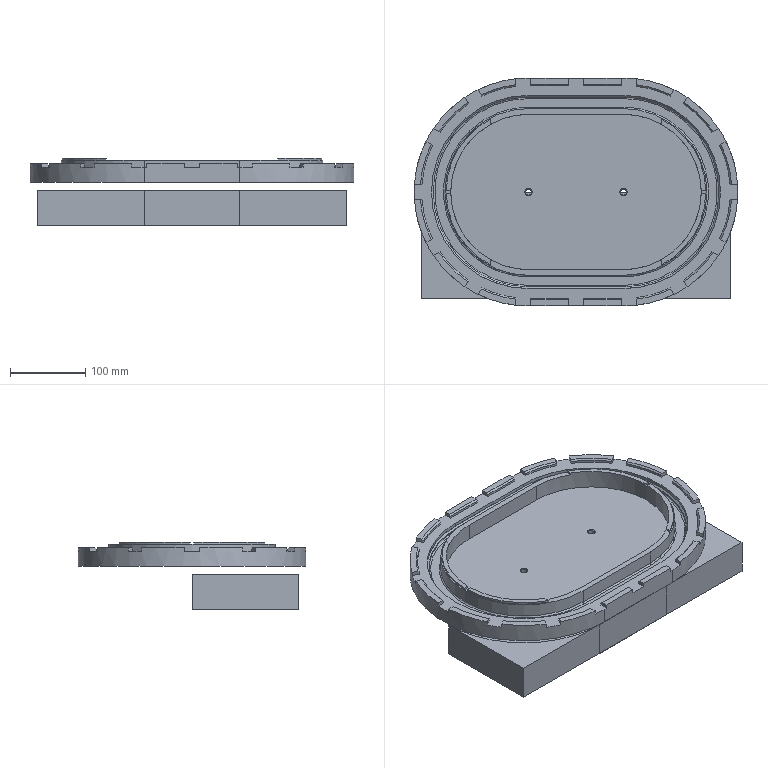NC program | NX | posted with a generic post | part box 429 x 302 x 89.371 mm
Lines 48932 to 50400 of 53366:
(PLANAR_MILL , TOOL : D63.)
N97854 T01 M6
N97856 G53
N97858 G17 G0 G90 X-190.948 Y-133.403 S4500 M3
N97860 G43 Z50. H1
N97862 Z3.1
N97864 G94 G1 Z0.1 F1500.
N97866 X-190.9 Y-70.403
N97868 G2 X-63.5 Y56.9 R127.4
N97870 G1 X63.5
N97872 G2 X190.9 Y-70.403 R127.4
N97874 G1 X190.948 Y-133.403
N97876 Z3.1
N97878 G0 Z50.
N97880 M5
(ADAPTIVE_MILLING_2 , TOOL : D16开粗)
N97882 T02 M6
N97884 G53
N97886 G17 G0 G90 X-224.171 Y-82.61 S6500 M3
N97888 G43 Z50. H2
N97890 Z-47.15
N97892 G94 G1 X-224.022 Y-82.588 Z-48.087 F3000.
N97894 X-223.874 Y-82.566 Z-48.458
N97896 X-223.725 Y-82.545 Z-48.73
N97898 X-223.577 Y-82.523 Z-48.95
N97900 X-223.429 Y-82.501 Z-49.134
N97902 X-223.28 Y-82.479 Z-49.292
N97904 X-223.132 Y-82.457 Z-49.43
N97906 X-222.983 Y-82.435 Z-49.55
N97908 X-222.835 Y-82.413 Z-49.655
N97910 X-222.687 Y-82.392 Z-49.748
N97912 X-222.538 Y-82.37 Z-49.829
N97914 X-222.39 Y-82.348 Z-49.9
N97916 X-222.241 Y-82.326 Z-49.96
N97918 X-222.093 Y-82.304 Z-50.012
N97920 X-221.945 Y-82.282 Z-50.055
N97922 X-221.796 Y-82.26 Z-50.089
N97924 X-221.648 Y-82.238 Z-50.116
N97926 X-221.499 Y-82.217 Z-50.135
N97928 X-221.351 Y-82.195 Z-50.146
N97930 X-221.203 Y-82.173 Z-50.15
N97932 X-218.756 Y-81.812
N97934 G3 X-217.377 Y-80.294 R1.616
N97936 G1 X-217.33 Y-79.346
N97938 G3 X-216.572 Y-73.312 R29.306
N97940 X-216.406 Y-60.427 R336.586
N97942 G1 X-216.401 Y-53.236
N97944 X-216.4 Y71.713
N97946 G2 X-214.045 Y77.327 R8.531
N97948 X-208.506 Y80.787 R13.167
N97950 X-201.742 Y82.057 R28.226
N97952 X-191.324 Y82.379 R143.598
N97954 G1 X-179.699 Y82.399
N97956 X205.701
N97958 G2 X211.373 Y80.002 R8.548
N97960 X214.807 Y74.446 R13.234
N97962 X216.043 Y67.902 R28.051
N97964 X216.374 Y58.01 R132.54
N97966 G1 X216.399 Y45.56
N97968 X216.4 Y-74.626
N97970 G3 X216.43 Y-76.436 R16.956
N97972 G1 X216.538 Y-76.795
N97974 G3 X217.249 Y-77.422 R1.606
N97976 G1 X218.397 Y-77.937
N97978 X221.284 Y-79.232 Z-50.05
N97980 X222.24 Y-79.661 F15000.
N97982 G3 X223.658 Y-76.795 R1.6
N97984 X222.224 Y-76.639 R1.659
N97986 X221.227 Y-77.757 R1.601
N97988 G1 X221.129 Y-78.154
N97990 X220.506 Y-80.674 Z-50.132 F3000.
N97992 G2 X220.252 Y-81.179 Z-50.15 R1.628
N97994 X217.377 Y-80.293 R1.6
N97996 G1 X217.33 Y-79.348
N97998 X217.049 Y-78.058
N98000 G3 X216.45 Y-76.634 R13.354
N98002 G2 X215.994 Y-73.564 R13.236
N98004 X215.806 Y-63.419 R183.776
N98006 G1 X215.8 Y-55.783
N98008 X215.799 Y46.392
N98010 G3 X215.672 Y63.09 R605.854
N98012 X214.951 Y70.698 R48.69
N98014 X213.141 Y75.758 R15.545
N98016 X207.97 Y80.015 R11.123
N98018 X201.787 Y81.461 R20.911
N98020 X193.696 Y81.776 R93.362
N98022 G1 X183.121 Y81.799
N98024 X-183.604 Y81.797
N98026 G3 X-198.002 Y81.638 R400.341
N98028 X-205.298 Y80.826 R42.086
N98030 X-210.087 Y78.934 R14.28
N98032 X-214.129 Y73.746 R11.263
N98034 X-215.472 Y67.766 R21.283
N98036 X-215.78 Y59.45 R97.239
N98038 G1 X-215.8 Y49.7
N98040 X-215.802 Y-55.212
N98042 G2 X-215.933 Y-71.609 R576.074
N98044 X-216.291 Y-76.26 R40.051
N98046 G1 X-216.426 Y-76.609
N98048 G2 X-217.715 Y-77.39 R1.601
N98050 G1 X-218.015 Y-77.379 Z-50.141
N98052 X-218.312 Y-77.339 Z-50.131
N98054 X-220.853 Y-77. Z-50.05
N98056 X-221.994 Y-76.848 F15000.
N98058 G2 X-223.303 Y-74.766 R1.6
N98060 X-223.056 Y-74.152 R2.69
N98062 X-220.094 Y-75.032 R1.6
N98064 G1 X-220.119 Y-76.281 Z-50.089 F3000.
N98066 X-220.13 Y-77.53 Z-50.129
N98068 G3 X-219.969 Y-78.171 Z-50.15 R1.61
N98070 X-217.049 Y-78.055 R1.6
N98072 G1 X-216.558 Y-76.829
N98074 G3 X-215.634 Y-74.452 R6.442
N98076 X-214.996 Y-68.51 R36.54
N98078 X-214.806 Y-53.902 R374.425
N98080 G1 X-214.801 Y-45.886
N98082 X-214.799 Y51.564
N98084 G2 X-214.65 Y63.937 R298.006
N98086 X-213.833 Y70.02 R29.015
N98088 X-208.514 Y77.163 R12.11
N98090 X-201.754 Y79.768 R19.619
N98092 X-193.408 Y80.633 R52.225
N98094 X-177.96 Y80.796 R457.105
N98096 G1 X183.44 Y80.798
N98098 G2 X197.239 Y80.676 R415.194
N98100 X203.487 Y79.955 R33.348
N98102 X211.258 Y74.357 R12.174
N98104 X213.758 Y67.797 R19.757
N98106 X214.619 Y59.752 R50.757
N98108 X214.795 Y46.254 R369.293
N98110 G1 X214.799 Y39.804
N98112 X214.801 Y-58.283
N98114 G3 X214.929 Y-71.046 R367.278
N98116 X215.302 Y-74.797 R25.132
N98118 X215.875 Y-75.701 R2.188
N98120 G1 X216.536 Y-76.792
N98122 X215.875 Y-75.701
N98124 G2 X215.03 Y-74.199 R2.937
N98126 X214.546 Y-71.334 R16.45
N98128 G1 X214.6 Y-70.393
N98130 X214.479 Y-64.464
N98132 G2 X214.212 Y-55.003 R131.
N98134 G1 X214.2 Y-44.608
N98136 X214.198 Y42.867
N98138 G3 X214.037 Y58.615 R473.699
N98140 X213.213 Y66.74 R52.179
N98142 X210.87 Y73.032 R18.805
N98144 X204.405 Y78.302 R13.292
N98146 X197.623 Y79.824 R24.476
N98148 X188.707 Y80.173 R102.828
N98150 G1 X178.208 Y80.198
N98152 X74.27
N98154 X69.43 Y80.484
N98156 X63.5 Y80.6
N98158 X-63.5
N98160 X-69.429 Y80.484
N98162 G2 X-79.045 Y80.211 R132.977
N98164 G1 X-89.442 Y80.199
N98166 X-176.992 Y80.197
N98168 G3 X-192.515 Y80.041 R478.334
N98170 X-200.715 Y79.22 R52.783
N98172 X-207.017 Y76.885 R18.876
N98174 X-212.301 Y70.434 R13.262
N98176 X-213.812 Y63.8 R24.137
N98178 X-214.175 Y54.66 R101.371
N98180 G1 X-214.2 Y43.41
N98182 X-214.202 Y-49.661
N98184 X-214.234 Y-60.343
N98186 X-214.479 Y-64.463
N98188 G2 X-214.65 Y-70.764 R154.546
N98190 X-215.372 Y-74.996 R18.001
N98192 X-215.873 Y-75.699 R2.633
N98194 G1 X-216.262 Y-76.341
N98196 G2 X-215.355 Y-75.098 R5.479
N98198 G3 X-214.388 Y-72.601 R5.961
N98200 X-214.533 Y-71.566 R5.627
N98202 G2 X-214.582 Y-69.492 R15.706
N98204 G3 X-214.36 Y-72.569 R11.764
N98206 G2 X-214.788 Y-74.431 R3.497
N98208 G1 X-214.973 Y-74.666
N98210 G2 X-217.856 Y-73.342 R1.76
N98212 G1 X-217.864 Y-72.984
N98214 X-217.857 Y-72.626
N98216 G2 X-214.371 Y-72.495 R1.76
N98218 X-214.647 Y-74.328 R2.312
N98220 G1 X-214.842 Y-74.556
N98222 G2 X-217.777 Y-73.31 R1.764
N98224 X-214.331 Y-72.725 R1.76
N98226 X-215.011 Y-74.698 R1.712
N98228 G1 X-215.403 Y-75.153
N98230 X-215.011 Y-74.698
N98232 G3 X-214.464 Y-74.11 R2.132
N98234 X-214.257 Y-73.038 R1.742
N98236 G2 X-214.6 Y-70.392 R11.715
N98238 G1 X-214.479 Y-64.463
N98240 X-214.126 Y-58.543
N98242 G3 X-213.412 Y-50.882 R227.461
N98244 X-213.208 Y-38.524 R257.535
N98246 G1 X-213.201 Y-29.686
N98248 X-213.199 Y46.089
N98250 G2 X-213.045 Y59.287 R338.024
N98252 X-212.162 Y66.345 R36.141
N98254 X-204.755 Y75.906 R14.381
N98256 X-197.439 Y78.283 R23.853
N98258 X-188.18 Y79.065 R67.153
N98260 X-168.981 Y79.198 R762.625
N98262 G1 X-87.017 Y79.2
N98264 X-83.742 Y79.209
N98266 X-81.252 Y79.554
N98268 X-75.35 Y80.135
N98270 X-72.055 Y80.329
N98272 X-75.35 Y80.135
N98274 X-81.252 Y79.554
N98276 G2 X-86.829 Y78.824 R124.765
N98278 X-95.915 Y78.608 R139.288
N98280 G1 X-105.566 Y78.598
N98282 X-171.966 Y78.596
N98284 G3 X-188.614 Y78.428 R507.501
N98286 X-197.265 Y77.583 R58.631
N98288 X-204.229 Y75.115 R21.683
N98290 X-210.648 Y67.394 R14.948
N98292 X-212.195 Y60.305 R27.1
N98294 X-212.568 Y51.241 R105.45
N98296 G1 X-212.6 Y39.766
N98298 X-212.603 Y-34.434
N98300 G2 X-212.692 Y-46.586 R593.408
N98302 G1 X-213.541 Y-52.641
N98304 X-212.692 Y-46.586
N98306 G3 X-212.016 Y-42.652 R83.716
N98308 X-211.655 Y-34.765 R84.937
N98310 X-211.601 Y-19.711 R919.087
N98312 G1 X-211.599 Y41.439
N98314 G2 X-211.458 Y55.162 R405.895
N98316 X-210.634 Y62.758 R44.512
N98318 X-207.527 Y69.761 R17.196
N98320 X-200.409 Y75.001 R16.987
N98322 X-192.634 Y76.909 R30.713
N98324 X-182.307 Y77.516 R98.636
N98326 X-167.757 Y77.596 R823.948
N98328 G1 X-107.04 Y77.598
N98330 G3 X-93.176 Y77.653 R792.36
N98332 G1 X-87.126 Y78.741
N98334 X-85.789 Y78.926
N98336 X-87.126 Y78.741
N98338 G3 X-94.453 Y77.397 R260.849
N98340 G2 X-100.372 Y77.052 R50.758
N98342 X-112.167 Y76.998 R762.663
N98344 G1 X-166.542 Y76.997
N98346 G3 X-184.465 Y76.846 R638.851
N98348 X-193.798 Y76.035 R69.198
N98350 X-201.264 Y73.638 R24.872
N98352 X-209.027 Y64.62 R16.259
N98354 X-210.596 Y57.078 R29.863
N98356 X-210.976 Y46.738 R124.853
N98358 G1 X-211.001 Y36.238
N98360 X-211.003 Y-23.183
N98362 G2 X-211.151 Y-38.061 R465.759
N98364 G1 X-211.188 Y-38.703
N98366 G3 X-212.088 Y-43.218 R65.915
N98368 G2 X-211.188 Y-38.703 R65.915
N98370 G3 X-210.497 Y-35.31 R41.524
N98372 X-210.071 Y-27.614 R72.782
N98374 X-210.001 Y-11.686 R894.824
N98376 G1 X-210. Y37.239
N98378 G2 X-209.846 Y52.087 R427.257
N98380 X-208.966 Y60.129 R47.328
N98382 X-205.764 Y67.501 R18.752
N98384 X-198.378 Y73.139 R17.775
N98386 X-190.339 Y75.216 R31.199
N98388 X-180.091 Y75.891 R93.521
N98390 X-159.692 Y75.998 R997.414
N98392 G1 X-111.469 Y76.
N98394 G3 X-100.026 Y76.104 R344.956
N98396 G2 X-93.923 Y77.489 R148.315
N98398 G3 X-100.782 Y75.913 R146.352
N98400 G2 X-105.867 Y75.493 R34.186
N98402 X-118.916 Y75.398 R556.154
N98404 G1 X-163.641 Y75.396
N98406 G3 X-181.34 Y75.24 R627.834
N98408 X-191.121 Y74.397 R73.113
N98410 X-198.956 Y71.916 R26.553
N98412 X-207.367 Y62.17 R17.305
N98414 X-208.955 Y54.555 R31.3
N98416 X-209.367 Y44.366 R119.716
N98418 G1 X-209.4 Y32.966
N98420 X-209.402 Y-14.484
N98422 G2 X-209.564 Y-30.247 R467.227
N98424 G1 X-209.698 Y-32.441
N98426 G3 X-210.629 Y-36.163 R65.262
N98428 G2 X-209.698 Y-32.441 R65.262
N98430 G3 X-208.925 Y-28.995 R25.582
N98432 X-208.48 Y-21.376 R71.284
N98434 X-208.401 Y-5.162 R881.015
N98436 G1 X-208.4 Y33.864
N98438 G2 X-208.245 Y49.012 R453.35
N98440 X-207.364 Y57.431 R51.664
N98442 X-204.262 Y65.025 R20.4
N98444 X-196.498 Y71.281 R18.342
N98446 X-188.047 Y73.55 R31.672
N98448 X-177.653 Y74.274 R92.47
N98450 X-156.429 Y74.398 R990.797
N98452 G1 X-118.744 Y74.399
N98454 G3 X-105.897 Y74.541 R349.309
N98456 X-104.496 Y74.932 R10.596
N98458 G1 X-100.505 Y75.973
N98460 G3 X-106.337 Y74.388 R116.008
N98462 G2 X-111.244 Y73.917 R29.538
N98464 X-126.416 Y73.798 R511.913
N98466 G1 X-160.191 Y73.796
N98468 G3 X-178.414 Y73.636 R651.268
N98470 X-188.57 Y72.772 R77.263
N98472 X-196.571 Y70.31 R28.251
N98474 X-205.624 Y60.108 R18.094
N98476 X-207.324 Y52.134 R32.228
N98478 X-207.761 Y41.871 R118.714
N98480 G1 X-207.801 Y29.046
N98482 X-207.802 Y-7.959
N98484 G2 X-207.958 Y-23.437 R479.667
N98486 X-208.21 Y-27.122 R38.621
N98488 G3 X-209.169 Y-30.416 R60.274
N98490 G2 X-207.689 Y-25.379 R132.919
N98492 G3 X-207.019 Y-19.717 R32.133
N98494 X-206.807 Y-6.352 R299.166
N98496 G1 X-206.802 Y0.239
N98498 X-206.8 Y30.189
N98500 G2 X-206.645 Y46.162 R494.709
N98502 X-205.778 Y54.81 R55.985
N98504 X-202.78 Y62.604 R22.02
N98506 X-194.637 Y69.467 R18.874
N98508 X-186.363 Y71.816 R31.497
N98510 X-175.903 Y72.642 R85.732
N98512 X-156.629 Y72.796 R746.021
N98514 G1 X-127.815 Y72.797
N98516 G3 X-112.603 Y72.912 R543.442
N98518 X-110.713 Y73.029 R17.729
N98520 G2 X-106.081 Y74.452 R520.224
N98522 G3 X-111.222 Y72.863 R195.156
N98524 G2 X-115.546 Y72.363 R24.092
N98526 X-127.32 Y72.199 R285.13
N98528 G1 X-151.516 Y72.198
N98530 X-165.341 Y72.179
N98532 G3 X-179.436 Y71.863 R266.432
N98534 X-188.865 Y70.604 R54.591
N98536 X-196.842 Y67.236 R24.122
N98538 X-204.029 Y57.76 R18.879
N98540 X-205.724 Y49.554 R34.137
N98542 X-206.164 Y38.691 R128.866
N98544 G1 X-206.201 Y25.116
N98546 X-206.202 Y-2.483
N98548 G2 X-206.36 Y-17.738 R469.371
N98550 X-206.699 Y-22.338 R49.244
N98552 G3 X-207.745 Y-25.591 R59.997
N98554 G2 X-206.217 Y-20.927 R93.803
N98556 G3 X-205.489 Y-15.781 R26.843
N98558 X-205.212 Y-3.193 R223.645
N98560 G1 X-205.202 Y5.039
N98562 X-205.199 Y27.863
N98564 G2 X-205.033 Y43.762 R471.871
N98566 X-204.144 Y52.558 R57.797
N98568 X-201.133 Y60.509 R23.054
N98570 X-192.721 Y67.722 R19.398
N98572 X-184.091 Y70.188 R32.269
N98574 X-173.556 Y71.031 R87.329
N98576 X-153.983 Y71.195 R727.875
N98578 G1 X-132.84 Y71.197
N98580 G3 X-117.786 Y71.318 R510.791
N98582 X-115.171 Y71.485 R29.374
N98584 G1 X-110.988 Y72.928
N98586 X-115.708 Y71.308
N98588 G2 X-120.271 Y70.767 R24.318
N98590 X-132.045 Y70.599 R282.305
N98592 G1 X-148.516 Y70.597
N98594 X-160.716 Y70.585
N98596 G3 X-176.012 Y70.307 R334.793
N98598 X-185.688 Y69.187 R63.067
N98600 X-194.013 Y66.076 R26.717
N98602 X-202.291 Y55.897 R19.384
N98604 X-204.069 Y47.633 R34.226
N98606 X-204.547 Y37.448 R116.043
N98608 X-204.601 Y21.923 R940.74
N98610 G1 X-204.603 Y2.466
N98612 G2 X-204.788 Y-13.226 R417.08
N98614 X-205.19 Y-18.006 R40.306
N98616 G1 X-206.29 Y-21.17
N98618 G2 X-204.744 Y-16.849 R97.792
N98620 G3 X-203.947 Y-11.872 R23.813
N98622 X-203.622 Y-0.328 R172.983
N98624 G1 X-203.602 Y11.188
N98626 X-203.599 Y24.938
N98628 G2 X-203.435 Y41.137 R495.717
N98630 X-202.558 Y50.161 R61.642
N98632 X-199.637 Y58.234 R24.362
N98634 X-190.853 Y65.989 R19.851
N98636 X-182.093 Y68.532 R32.753
N98638 X-171.411 Y69.416 R86.981
N98640 X-152.213 Y69.594 R667.309
N98642 G1 X-146.438 Y69.597
N98644 X-134.121 Y69.598
N98646 G3 X-121.539 Y69.765 R296.389
N98648 X-119.178 Y69.951 R28.146
N98650 G1 X-115.421 Y71.392
N98652 X-119.573 Y69.801
N98654 G2 X-123.755 Y69.219 R20.828
N98656 X-133.416 Y69.008 R181.21
N98658 G1 X-145.366 Y68.997
N98660 X-157.491 Y68.985
N98662 G3 X-173.687 Y68.698 R352.113
N98664 X-183.585 Y67.548 R64.572
N98666 X-192.061 Y64.395 R27.516
N98668 X-200.569 Y54.063 R19.868
N98670 X-202.428 Y45.663 R34.413
N98672 X-202.943 Y35.105 R115.113
N98674 X-203.001 Y18.83 R962.629
N98676 G1 X-203.002 Y8.316
N98678 G2 X-203.172 Y-8.13 R488.09
N98680 X-203.695 Y-14.178 R49.533
N98682 G1 X-204.818 Y-17.068
N98684 X-203.202 Y-12.919
N98686 G3 X-202.371 Y-7.873 R24.034
N98688 X-202.027 Y3.28 R162.316
N98690 G1 X-202.002 Y13.289
N98692 X-201.994 Y26.314
N98694 G2 X-201.747 Y40.635 R301.013
N98696 X-200.629 Y49.478 R51.051
N98698 X-196.883 Y57.931 R22.784
N98700 X-188.327 Y64.584 R20.787
N98702 X-179.297 Y67.012 R35.189
N98704 X-168.234 Y67.837 R97.314
N98706 X-150.085 Y67.994 R724.413
N98708 G1 X-138.994 Y67.998
N98710 G3 X-126.158 Y68.155 R327.901
N98712 X-122.959 Y68.406 R34.652
N98714 X-121.298 Y69.109 R21.076
N98716 G1 X-119.273 Y69.901
N98718 G3 X-123.055 Y68.341 R60.652
N98720 G2 X-126.643 Y67.707 R15.561
N98722 X-135.763 Y67.418 R124.528
N98724 G1 X-142.244 Y67.398
N98726 X-152.118 Y67.39
N98728 G3 X-169.591 Y67.173 R504.845
N98730 X-180.112 Y66.19 R79.698
N98732 X-188.811 Y63.454 R31.272
N98734 X-198.97 Y51.959 R20.393
N98736 X-200.834 Y43.331 R35.867
N98738 X-201.35 Y32.097 R124.686
N98740 X-201.401 Y17.322 R917.732
N98742 G2 X-201.521 Y-2.212 R851.075
N98744 X-202.096 Y-10.038 R64.021
N98746 X-202.239 Y-10.712 R8.727
N98748 G3 X-203.259 Y-13.091 R198.496
N98750 G2 X-201.749 Y-9.563 R410.384
N98752 G3 X-200.867 Y-4.958 R20.592
N98754 X-200.448 Y5.113 R121.989
N98756 X-200.401 Y18.593 R879.379
N98758 G2 X-200.24 Y36.141 R583.583
N98760 X-199.35 Y45.767 R67.736
N98762 X-196.515 Y54.035 R26.296
N98764 X-187.14 Y62.595 R20.665
N98766 X-178.179 Y65.244 R33.674
N98768 X-167.202 Y66.193 R87.469
N98770 X-150.329 Y66.39 R547.236
N98772 G1 X-138.943 Y66.406
N98774 G3 X-128.374 Y66.66 R166.521
N98776 X-126.396 Y66.886 R13.005
N98778 G1 X-123.026 Y68.353
N98780 G2 X-126.828 Y66.711 R128.149
N98782 X-130.964 Y66.069 R19.423
N98784 X-140.776 Y65.812 R156.182
N98786 G1 X-153.925 Y65.779
N98788 G3 X-169.521 Y65.467 R324.698
N98790 X-179.565 Y64.277 R66.501
N98792 X-188.266 Y61.059 R28.805
N98794 X-197.315 Y50.057 R20.777
N98796 X-199.208 Y41.357 R36.383
N98798 X-199.748 Y29.824 R125.441
N98800 X-199.804 Y14.771 R949.656
N98802 G2 X-200.005 Y-0.517 R389.711
N98804 X-200.656 Y-7.057 R46.377
N98806 G1 X-201.845 Y-9.811
N98808 X-200.225 Y-6.16
N98810 G3 X-199.295 Y-1.479 R20.228
N98812 X-198.859 Y8.203 R114.559
N98814 X-198.791 Y22.676 R941.419
N98816 G2 X-198.501 Y36.847 R268.468
N98818 X-197.289 Y45.828 R50.795
N98820 X-193.335 Y54.503 R23.456
N98822 X-184.428 Y61.317 R21.673
N98824 X-175.397 Y63.744 R36.486
N98826 X-164.037 Y64.621 R98.148
N98828 X-144.786 Y64.798 R753.624
N98830 G3 X-133. Y65.008 R239.008
N98832 X-129.685 Y65.334 R34.604
N98834 G1 X-129.471 Y65.405
N98836 X-126.595 Y66.793
N98838 G2 X-129.901 Y65.218 R112.975
N98840 X-133.776 Y64.529 R16.952
N98842 X-143.047 Y64.218 R126.093
N98844 G1 X-155.689 Y64.156
N98846 G3 X-169.63 Y63.715 R216.395
N98848 X-179.404 Y62.224 R55.057
N98850 X-187.989 Y58.39 R26.309
N98852 X-195.658 Y48.207 R21.201
N98854 X-197.583 Y39.438 R36.847
N98856 X-198.132 Y28.656 R118.565
N98858 X-198.211 Y14.644 R886.867
N98860 G2 X-198.485 Y1.763 R247.823
N98862 X-199.202 Y-4.078 R36.658
N98864 G1 X-200.368 Y-6.512
N98866 G3 X-198.689 Y-2.997 R76.831
N98868 X-197.724 Y1.769 R20.59
N98870 X-197.259 Y11.805 R114.985
N98872 G1 X-197.171 Y24.493
N98874 G2 X-196.749 Y36.783 R169.005
N98876 X-195.185 Y45.629 R42.162
N98878 X-189.467 Y55.185 R21.938
N98880 X-180.685 Y60.401 R23.825
N98882 X-171.016 Y62.437 R44.207
N98884 X-158.513 Y63.097 R139.531
N98886 X-145.043 Y63.207 R873.644
N98888 G3 X-135.109 Y63.508 R142.537
N98890 X-132.747 Y63.809 R16.279
N98892 G1 X-129.639 Y65.324
N98894 G3 X-132.827 Y63.744 R81.853
N98896 G2 X-136.095 Y63.037 R13.113
N98898 X-144.228 Y62.64 R86.993
N98900 G1 X-156.089 Y62.528
N98902 G3 X-169.273 Y61.962 R167.746
N98904 X-178.921 Y60.189 R48.373
N98906 X-187.704 Y55.554 R24.669
N98908 X-194.139 Y46.013 R21.825
N98910 X-196.011 Y37.079 R38.672
N98912 X-196.546 Y25.545 R132.199
N98914 G1 X-196.641 Y13.722
N98916 G2 X-197.076 Y2.841 R135.263
N98918 X-197.699 Y-1.068 R24.751
N98920 G1 X-198.85 Y-3.387
N98922 G2 X-197.274 Y-0.266 R95.823
N98924 G3 X-196.25 Y4.048 R17.099
N98926 X-195.69 Y13.431 R91.645
N98928 G1 X-195.546 Y24.901
N98930 G2 X-194.997 Y36.284 R127.903
N98932 X-193.142 Y44.993 R37.524
N98934 X-181.671 Y57.606 R21.671
N98936 X-172.418 Y60.36 R35.097
N98938 X-161.07 Y61.37 R89.974
N98940 X-145.699 Y61.626 R687.881
N98942 G3 X-137.112 Y62.041 R90.965
N98944 X-135.497 Y62.321 R7.993
N98946 G1 X-132.716 Y63.8
N98948 G2 X-135.849 Y62.15 R81.169
N98950 X-139.602 Y61.4 R15.627
N98952 X-148.506 Y61.009 R108.717
N98954 G3 X-162.808 Y60.671 R400.598
N98956 X-173.455 Y59.468 R72.728
N98958 X-182.351 Y56.343 R31.11
N98960 X-192.309 Y44.707 R21.708
N98962 X-194.326 Y35.805 R37.206
N98964 X-194.929 Y24.801 R117.668
N98966 G2 X-195.18 Y10.917 R757.361
N98968 X-195.859 Y3.282 R59.072
N98970 X-196.246 Y1.625 R10.035
N98972 G1 X-197.378 Y-0.491
N98974 X-195.738 Y2.601
N98976 G3 X-194.696 Y6.872 R17.192
N98978 X-194.097 Y16.016 R86.761
N98980 G2 X-193.778 Y29.006 R669.856
N98982 X-192.719 Y38.764 R64.635
N98984 X-189.529 Y47.376 R27.073
N98986 X-179.843 Y55.976 R21.989
N98988 X-170.451 Y58.754 R35.683
N98990 X-159.029 Y59.768 R91.802
N98992 X-146.684 Y60.054 R891.975
N98994 G3 X-139.098 Y60.596 R63.068
N98996 X-138.18 Y60.836 R2.911
N98998 G2 X-135.58 Y62.27 R56.092
N99000 G3 X-138.374 Y60.722 R54.47
N99002 G2 X-141.465 Y59.936 R11.426
N99004 X-149.128 Y59.43 R73.261
N99006 G3 X-161.83 Y59.011 R399.882
N99008 X-172.384 Y57.675 R67.253
N99010 X-181.392 Y54.219 R29.851
N99012 X-190.633 Y43.006 R21.96
N99014 X-192.699 Y34.039 R37.347
N99016 X-193.348 Y22.737 R122.298
N99018 G2 X-193.746 Y10.929 R263.723
N99020 X-194.656 Y4.565 R35.248
N99022 X-195.299 Y3.394 R8.18
N99024 G1 X-195.829 Y2.402
N99026 G2 X-194.303 Y5.114 R87.681
N99028 G3 X-193.21 Y9.1 R15.207
N99030 X-192.53 Y17.383 R72.629
N99032 G2 X-192.095 Y28.716 R486.168
N99034 X-190.828 Y38.145 R55.89
N99036 X-186.995 Y46.977 R25.487
N99038 X-177.578 Y54.556 R22.597
N99040 X-168.211 Y57.198 R37.191
N99042 X-156.861 Y58.182 R97.468
N99044 G3 X-146.363 Y58.567 R669.582
N99046 X-141.129 Y59.168 R36.95
N99048 G1 X-140.824 Y59.287
N99050 X-138.364 Y60.728
N99052 G2 X-141.241 Y59.07 R54.196
N99054 X-144.864 Y58.255 R14.858
N99056 X-152.207 Y57.761 R91.905
N99058 G3 X-163.729 Y57.107 R192.532
N99060 X-173.444 Y55.289 R49.869
N99062 X-182.502 Y50.523 R25.651
N99064 X-189.208 Y40.66 R22.638
N99066 X-191.16 Y31.588 R39.869
N99068 X-191.759 Y22.084 R131.264
N99070 G2 X-192.318 Y11.89 R158.321
N99072 X-193.184 Y7.035 R27.312
N99074 X-194.389 Y4.945 R38.712
N99076 G1 X-192.744 Y7.775
N99078 G3 X-191.591 Y12.037 R16.271
N99080 X-190.884 Y20.099 R81.055
N99082 G2 X-190.245 Y30.036 R193.619
N99084 X-188.498 Y38.847 R42.099
N99086 X-182.048 Y48.938 R22.811
N99088 X-172.98 Y54.014 R25.553
N99090 X-163.147 Y56.018 R47.884
N99092 X-152.159 Y56.752 R181.069
N99094 G3 X-144.706 Y57.406 R67.884
N99096 X-143.41 Y57.723 R4.92
N99098 G2 X-140.994 Y59.188 R62.556
N99100 G3 X-143.535 Y57.639 R51.936
N99102 G2 X-146.436 Y56.8 R10.5
N99104 X-153.201 Y56.137 R65.689
N99106 G3 X-163.654 Y55.304 R164.139
N99108 X-173.356 Y53.086 R43.7
N99110 X-182.676 Y47.075 R23.965
N99112 X-187.976 Y37.712 R23.971
N99114 X-189.716 Y28.365 R46.125
N99116 X-190.383 Y18.469 R333.251
N99118 G2 X-191.26 Y11.091 R53.91
N99120 X-191.734 Y9.394 R8.996
N99122 G3 X-192.867 Y7.539 R69.572
N99124 G2 X-191.303 Y10.083 R89.229
N99126 G3 X-190.107 Y13.978 R14.329
N99128 X-189.252 Y21.554 R74.308
N99130 G2 X-188.311 Y30.95 R120.725
N99132 X-185.814 Y39.805 R33.71
N99134 X-174.705 Y50.987 R22.592
N99136 X-165.32 Y53.848 R36.401
N99138 X-155.111 Y54.979 R101.649
N99140 G3 X-147.617 Y55.729 R85.878
N99142 X-145.938 Y56.113 R8.255
N99144 G1 X-143.498 Y57.663
N99146 X-146.025 Y56.046
N99148 G2 X-149.06 Y55.14 R11.153
N99150 X-156.037 Y54.328 R82.591
N99152 G3 X-165.776 Y53.073 R91.008
N99154 X-174.999 Y49.942 R33.635
N99156 X-185.718 Y37.783 R22.732
N99158 X-187.86 Y29.057 R38.913
N99160 X-188.785 Y19.936 R196.689
N99162 G2 X-189.798 Y13.102 R48.168
N99164 X-190.234 Y11.729 R6.79
N99166 G1 X-191.408 Y9.897
N99168 X-189.693 Y12.602
N99170 G3 X-188.446 Y16.654 R15.816
N99172 X-187.48 Y23.759 R96.2
N99174 G2 X-186.071 Y32.566 R70.314
N99176 X-182.355 Y41.379 R27.347
N99178 X-172.523 Y49.566 R23.146
N99180 X-163.259 Y52.304 R38.32
N99182 X-154.102 Y53.488 R145.092
N99184 G3 X-148.613 Y54.394 R39.404
N99186 G1 X-148.276 Y54.556
N99188 G2 X-146.023 Y56.047 R53.256
N99190 G3 X-148.461 Y54.428 R51.907
N99192 G2 X-151.266 Y53.493 R10.474
N99194 X-158.099 Y52.449 R91.879
N99196 G3 X-167.011 Y50.762 R64.759
N99198 X-176.029 Y46.613 R28.536
N99200 X-184.088 Y36.112 R23.078
N99202 X-186.285 Y27.635 R40.382
N99204 X-187.4 Y19.556 R630.684
N99206 G2 X-188.544 Y14.362 R30.269
N99208 X-189.098 Y13.503 R5.156
N99210 G1 X-189.826 Y12.366
N99212 G2 X-188.183 Y14.838 R96.061
N99214 G3 X-186.848 Y18.667 R14.785
N99216 X-185.588 Y25.681 R125.538
N99218 G2 X-183.62 Y33.838 R48.941
N99220 X-177.532 Y43.47 R23.974
N99222 X-168.352 Y48.944 R25.952
N99224 X-159.622 Y51.095 R50.596
N99226 G3 X-152.768 Y52.258 R199.701
N99228 X-150.875 Y52.762 R10.589
N99230 G1 X-148.406 Y54.466
N99232 X-150.929 Y52.708
N99234 G2 X-153.933 Y51.64 R11.625
N99236 X-160.695 Y50.285 R193.456
N99238 G3 X-169.389 Y47.736 R44.048
N99240 X-179.168 Y40.324 R23.967
N99242 X-183.511 Y31.552 R27.1
N99244 X-185.198 Y24.095 R67.45
N99246 G2 X-186.529 Y17.87 R64.919
N99248 X-187.034 Y16.46 R8.016
N99250 G1 X-188.322 Y14.615
N99252 X-186.464 Y17.301
N99254 G3 X-185.008 Y21.229 R17.079
N99256 X-183.428 Y27.78 R767.859
N99258 G2 X-180.47 Y35.79 R35.45
N99260 X-169.731 Y46.048 R23.723
N99262 X-161.223 Y48.972 R40.744
N99264 G3 X-154.809 Y50.463 R322.418
N99266 X-153.392 Y50.933 R6.549
N99268 G2 X-150.925 Y52.711 R63.888
N99270 G3 X-153.509 Y50.838 R52.784
N99272 G2 X-156.554 Y49.622 R12.845
N99274 G3 X-163.037 Y47.843 R894.797
N99276 X-171.478 Y44.17 R33.752
N99278 X-180.675 Y33.429 R24.045
N99280 X-183.172 Y25.961 R46.481
N99282 G2 X-184.816 Y20.025 R85.403
N99284 X-185.704 Y18.367 R4.022
N99286 G1 X-186.563 Y17.136
N99288 G2 X-184.701 Y19.71 R80.345
N99290 G3 X-183.087 Y23.401 R18.015
N99292 G2 X-180.975 Y29.689 R202.518
N99294 X-176.399 Y37.925 R28.833
N99296 X-167.182 Y44.908 R25.615
N99298 X-159.989 Y47.525 R54.287
N99300 G3 X-156.337 Y48.724 R47.626
N99302 X-153.488 Y50.853 R65.407
N99304 G2 X-156.618 Y48.509 R91.058
N99306 X-160.325 Y46.916 R23.807
N99308 G3 X-166.907 Y44.248 R64.296
N99310 X-179.114 Y32.011 R25.61
N99312 X-181.867 Y25.053 R64.245
N99314 G2 X-183.188 Y21.694 R30.914
N99316 G1 X-184.806 Y19.553
N99318 G3 X-182.332 Y22.858 R85.712
N99320 X-180.232 Y27.107 R35.687
N99322 G2 X-176.686 Y33.896 R45.392
N99324 X-166.557 Y42.936 R26.86
N99326 X-160.295 Y45.774 R76.576
N99328 G3 X-159.465 Y46.176 R6.068
N99330 G2 X-156.411 Y48.642 R82.885
N99332 G3 X-159.908 Y45.83 R181.941
N99334 G2 X-162.801 Y44.197 R27.829
N99336 G3 X-169.031 Y40.587 R49.22
N99338 X-177.423 Y31.135 R28.206
N99340 X-180.31 Y25.456 R125.497
N99342 G1 X-180.578 Y24.975
N99344 G3 X-182.576 Y22.496 R72.977
N99346 G2 X-179.327 Y26.511 R167.382
N99348 G3 X-176.357 Y31.011 R161.669
N99350 G2 X-165.698 Y41.227 R32.508
N99352 G1 X-164.094 Y42.209
N99354 G2 X-159.681 Y45.998 R91.11
N99356 G3 X-164.094 Y42.209 R91.11
N99358 G2 X-167.802 Y39.158 R62.773
N99360 G3 X-175.802 Y30.551 R38.962
N99362 X-179.454 Y26.344 R98.236
N99364 G2 X-175.802 Y30.551 R98.236
N99366 G1 X-174.418 Y32.108
N99368 X-170.306 Y36.382
N99370 X-166.029 Y40.491
N99372 X-165.02 Y41.387
N99374 G3 X-164.751 Y43.497 R1.616
N99376 G1 X-166.19 Y45.639
N99378 X-166.274 Y45.763 Z-50.146
N99380 X-166.357 Y45.888 Z-50.135
N99382 X-166.441 Y46.012 Z-50.116
N99384 X-166.524 Y46.137 Z-50.089
N99386 X-166.608 Y46.261 Z-50.055
N99388 X-166.692 Y46.386 Z-50.012
N99390 X-166.775 Y46.51 Z-49.96
N99392 X-166.859 Y46.635 Z-49.9
N99394 X-166.943 Y46.759 Z-49.829
N99396 X-167.026 Y46.884 Z-49.748
N99398 X-167.11 Y47.008 Z-49.655
N99400 X-167.193 Y47.133 Z-49.55
N99402 X-167.277 Y47.257 Z-49.43
N99404 X-167.361 Y47.382 Z-49.292
N99406 X-167.444 Y47.506 Z-49.134
N99408 X-167.528 Y47.631 Z-48.95
N99410 X-167.612 Y47.755 Z-48.73
N99412 X-167.695 Y47.88 Z-48.458
N99414 X-167.779 Y48.005 Z-48.087
N99416 X-167.863 Y48.129 Z-47.15
N99418 G0 Z50.
N99420 X75.55 Y84.086
N99422 Z-47.15
N99424 G1 X75.4 Y84.094 Z-48.087
N99426 X75.25 Y84.103 Z-48.458
N99428 X75.101 Y84.112 Z-48.73
N99430 X74.951 Y84.121 Z-48.95
N99432 X74.801 Y84.13 Z-49.134
N99434 X74.651 Y84.138 Z-49.292
N99436 X74.502 Y84.147 Z-49.43
N99438 X74.352 Y84.156 Z-49.55
N99440 X74.202 Y84.165 Z-49.655
N99442 X74.052 Y84.174 Z-49.748
N99444 X73.903 Y84.183 Z-49.829
N99446 X73.753 Y84.191 Z-49.9
N99448 X73.603 Y84.2 Z-49.96
N99450 X73.454 Y84.209 Z-50.012
N99452 X73.304 Y84.218 Z-50.055
N99454 X73.154 Y84.227 Z-50.089
N99456 X73.004 Y84.236 Z-50.116
N99458 X72.855 Y84.244 Z-50.135
N99460 X72.705 Y84.253 Z-50.146
N99462 X72.555 Y84.262 Z-50.15
N99464 G3 X71.81 Y81.169 R1.616
N99466 G1 X73.714 Y80.332
N99468 G3 X74.27 Y80.198 R1.681
N99470 G1 X75.35 Y80.135
N99472 G3 X83.191 Y79.408 R238.599
N99474 X94.881 Y79.208 R248.587
N99476 G1 X104.763 Y79.198
N99478 X180.163 Y79.197
N99480 G2 X193.287 Y79.042 R331.852
N99482 X200.344 Y78.155 R36.096
N99484 X209.978 Y70.611 R14.416
N99486 X212.322 Y63.2 R24.273
N99488 X213.064 Y54.238 R68.309
N99490 X213.199 Y35.039 R753.222
N99492 G1 X213.2 Y-42.824
N99494 X213.209 Y-50.254
N99496 X213.541 Y-52.642
N99498 X214.126 Y-58.544
N99500 X214.332 Y-61.987
N99502 X214.126 Y-58.544
N99504 X213.541 Y-52.642
N99506 G2 X212.841 Y-47.391 R149.109
N99508 X212.613 Y-38.755 R123.374
N99510 G1 X212.6 Y-28.634
N99512 X212.598 Y37.466
N99514 G3 X212.436 Y54.414 R540.661
N99516 X211.591 Y63.216 R59.559
N99518 X209.173 Y70.122 R21.863
N99520 X201.3 Y76.677 R14.987
N99522 X194.132 Y78.208 R27.535
N99524 X184.317 Y78.575 R116.21
N99526 G1 X174.492 Y78.598
N99528 X99.717 Y78.601
N99530 G2 X87.412 Y78.691 R602.949
N99532 G1 X81.252 Y79.554
N99534 X87.412 Y78.691
N99536 G3 X91.529 Y77.996 R68.603
N99538 X100.258 Y77.637 R99.284
N99540 G1 X114.438 Y77.599
N99542 X175.438 Y77.597
N99544 G2 X189.462 Y77.442 R381.68
N99546 X197.05 Y76.561 R42.177
N99548 X204.168 Y73.192 R16.8
N99550 X209.128 Y66.082 R17.313
N99552 X210.978 Y58.061 R32.129
N99554 X211.531 Y47.43 R110.291
N99556 X211.599 Y31.23 R928.059
N99558 G1 Y-26.785
N99560 G3 X211.653 Y-40.804 R853.23
N99562 G1 X212.725 Y-46.768
N99564 X212.921 Y-48.179
N99566 X212.725 Y-46.768
N99568 G3 X211.404 Y-39.582 R265.2
N99570 G2 X211.055 Y-33.675 R50.208
N99572 X210.999 Y-21.883 R759.325
N99574 G1 X210.997 Y33.567
N99576 G3 X210.828 Y50.965 R554.979
N99578 X209.986 Y60.068 R65.427
N99580 X207.503 Y67.506 R24.253
N99582 X198.623 Y75.018 R16.266
N99584 X191.08 Y76.591 R29.857
N99586 X180.74 Y76.973 R124.226
N99588 G1 X170.24 Y76.998
N99590 X110.742 Y77.
N99592 G2 X95.732 Y77.159 R432.491
N99594 G1 X95.299 Y77.187
N99596 G3 X90.75 Y78.095 R66.302
N99598 G2 X95.299 Y77.187 R66.302
N99600 G3 X98.871 Y76.473 R39.715
N99602 X106.966 Y76.057 R78.96
N99604 X122.313 Y75.999 R908.213
N99606 G1 X171.313 Y75.997
N99608 G2 X186.162 Y75.84 R418.159
N99610 X194.203 Y74.943 R46.666
N99612 X201.509 Y71.749 R18.694
N99614 X207.203 Y64.216 R17.841
N99616 X209.258 Y56.015 R31.822
N99618 X209.907 Y45.315 R100.654
N99620 X209.997 Y29.865 R842.116
N99622 G1 X209.999 Y-18.536
N99624 G3 X210.093 Y-33.87 R638.504
N99626 X210.404 Y-35.138 R23.704
N99628 G1 X211.484 Y-40.046
N99630 G3 X209.911 Y-33.204 R151.897
N99632 G2 X209.493 Y-28.11 R34.395
N99634 X209.399 Y-15.059 R562.746
N99636 G1 X209.397 Y29.666
N99638 G3 X209.236 Y47.44 R615.354
N99640 X208.391 Y57.146 R72.598
N99642 X205.968 Y64.843 R26.582
N99644 X196.297 Y73.314 R17.277
N99646 X188.462 Y74.96 R31.291
N99648 X178.424 Y75.364 R120.308
N99650 G1 X165.674 Y75.398
N99652 X119.516 Y75.399
N99654 G2 X104.248 Y75.542 R506.161
N99656 X101.55 Y75.701 R47.368
N99658 G3 X97.806 Y76.638 R67.81
N99660 G2 X103.582 Y75.171 R142.568
N99662 G3 X109.139 Y74.585 R35.471
N99664 X123.893 Y74.401 R378.877
N99666 G1 X128.838 Y74.399
N99668 X167.863 Y74.397
N99670 G2 X183.087 Y74.24 R446.282
N99672 X191.431 Y73.358 R51.325
N99674 X198.893 Y70.346 R20.549
N99676 X205.309 Y62.427 R18.344
N99678 X207.528 Y54.194 R31.565
N99680 X208.263 Y44.101 R88.992
N99682 X208.397 Y25.952 R779.159
N99684 G1 X208.399 Y-12.61
N99686 G3 X208.523 Y-27.722 R493.16
N99688 X208.582 Y-28.343 R10.199
N99690 G2 X209.966 Y-33.464 R112.79
N99692 G3 X208.386 Y-27.653 R118.963
N99694 G2 X207.917 Y-22.733 R29.675
N99696 X207.799 Y-7.559 R517.293
N99698 G1 X207.797 Y25.916
N99700 G3 X207.628 Y44.664 R640.361
N99702 X206.791 Y54.447 R76.793
N99704 X204.396 Y62.389 R28.6
N99706 X194.025 Y71.648 R18.125
N99708 X186.045 Y73.329 R32.572
N99710 X175.932 Y73.758 R119.081
N99712 X163.183 Y73.798 R854.614
N99714 G1 X126.041 Y73.799
N99716 G2 X110.352 Y73.964 R457.737
N99718 X106.878 Y74.21 R34.779
N99720 G3 X103.553 Y75.178 R62.799
N99722 G2 X108.529 Y73.709 R117.738
N99724 G3 X114.008 Y73.031 R30.308
N99726 X126.005 Y72.808 R249.129
N99728 G1 X135.738 Y72.799
N99730 X165.088 Y72.797
N99732 G2 X180.386 Y72.633 R445.445
N99734 X189.103 Y71.714 R53.723
N99736 X196.801 Y68.643 R21.644
N99738 X203.566 Y60.41 R18.97
N99740 X205.874 Y51.97 R32.369
N99742 X206.659 Y41.355 R90.932
N99744 X206.797 Y23.356 R775.963
N99746 G1 X206.798 Y-6.085
N99748 G3 X206.916 Y-21.446 R532.82
N99750 X207.046 Y-23.345 R12.328
N99752 G1 X208.465 Y-27.96
N99754 G2 X206.822 Y-22.593 R477.404
N99756 X206.327 Y-17.615 R29.605
N99758 X206.199 Y-4.184 R413.602
N99760 G1 X206.197 Y22.766
N99762 G3 X206.033 Y41.665 R680.834
N99764 X205.192 Y51.899 R82.207
N99766 X202.737 Y60.217 R30.19
N99768 X191.826 Y69.999 R18.85
N99770 X183.7 Y71.705 R33.768
N99772 X172.688 Y72.162 R126.426
N99774 G1 X159.188 Y72.198
N99776 X131.517 Y72.2
N99778 G2 X115.841 Y72.374 R435.073
N99780 X111.701 Y72.688 R53.693
N99782 G3 X108.522 Y73.712 R63.683
N99784 G2 X113.077 Y72.214 R93.72
N99786 G3 X118.286 Y71.482 R26.961
N99788 X129.168 Y71.216 R196.72
N99790 G1 X139.039 Y71.199
N99792 X162.013 Y71.196
N99794 G2 X177.836 Y71.027 R458.711
N99796 X186.705 Y70.11 R56.854
N99798 X194.702 Y67.003 R22.796
N99800 X201.833 Y58.47 R19.532
N99802 X204.217 Y49.895 R32.873
N99804 X205.037 Y39.358 R89.433
N99806 X205.197 Y19.709 R753.044
N99808 G1 X205.198 Y-1.135
N99810 G3 X205.327 Y-16.399 R488.237
N99812 X205.497 Y-18.879 R21.599
N99814 G1 X206.961 Y-23.101
N99816 X205.315 Y-18.321
N99818 G2 X204.779 Y-13.901 R23.833
N99820 X204.6 Y-1.93 R266.284
N99822 G1 X204.599 Y14.391
N99824 X204.586 Y26.591
N99826 G3 X204.314 Y41.888 R340.896
N99828 X203.212 Y51.565 R64.024
N99830 X200.173 Y59.844 R26.995
N99832 X189.999 Y68.248 R19.363
N99834 X181.816 Y70.046 R33.738
N99836 X171.407 Y70.545 R113.994
N99838 X156.032 Y70.598 R933.49
N99840 G1 X136.466 Y70.6
N99842 G2 X120.796 Y70.783 R421.078
N99844 X116.005 Y71.186 R41.576
N99846 G1 X112.87 Y72.276
N99848 G2 X117.155 Y70.741 R91.122
N99850 G3 X121.995 Y69.954 R23.365
N99852 X133.449 Y69.62 R167.055
N99854 G1 X144.963 Y69.599
N99856 X158.863 Y69.597
N99858 G2 X175.137 Y69.432 R496.87
N99860 X184.382 Y68.51 R60.458
N99862 X192.422 Y65.519 R23.983
N99864 X200.098 Y56.613 R19.973
N99866 X202.584 Y47.755 R33.489
N99868 X203.439 Y36.695 R92.497
N99870 X203.596 Y18.021 R739.147
N99872 G1 X203.598 Y3.44
N99874 G3 X203.737 Y-11.88 R463.163
N99876 X203.961 Y-14.863 R24.82
N99878 G2 X205.404 Y-18.62 R248.091
N99880 G3 X203.873 Y-14.656 R177.74
N99882 G2 X203.259 Y-10.807 R17.029
N99884 X203.009 Y-0.633 R160.179
N99886 G1 X202.998 Y11.691
N99888 X202.986 Y23.816
N99890 G3 X202.708 Y39.487 R350.334
N99892 X201.588 Y49.389 R66.142
N99894 X198.534 Y57.819 R27.941
N99896 X187.994 Y66.589 R19.876
N99898 X179.739 Y68.415 R34.465
N99900 X169.256 Y68.938 R112.945
N99902 X153.806 Y68.998 R917.446
N99904 G1 X142.166 Y68.999
N99906 G2 X125.799 Y69.172 R478.765
N99908 X119.854 Y69.685 R50.205
N99910 G1 X116.943 Y70.812
N99912 G3 X121.289 Y69.139 R106.265
N99914 X126.459 Y68.342 R26.112
N99916 X137.28 Y68.024 R170.016
N99918 G1 X147.289 Y67.999
N99920 X157.064 Y67.996
N99922 G2 X173.112 Y67.815 R458.144
N99924 X182.354 Y66.867 R60.637
N99926 X190.605 Y63.776 R24.577
N99928 X198.374 Y54.79 R20.393
N99930 X200.936 Y45.795 R33.891
N99932 X201.83 Y34.512 R92.582
N99934 X201.994 Y16.438 R688.335
N99936 G1 X201.999 Y4.945
N99938 G3 X202.165 Y-8.091 R322.199
N99940 X202.406 Y-11.045 R29.714
N99942 X203.068 Y-12.603 R28.392
N99944 G1 X203.889 Y-14.697
N99946 G3 X202.283 Y-10.77 R122.869
N99948 G2 X201.67 Y-6.895 R18.115
N99950 X201.409 Y3.716 R163.065
N99952 G1 X201.398 Y11.319
N99954 X201.365 Y25.544
N99956 G3 X200.947 Y39.71 R221.795
N99958 X199.507 Y49.264 R53.511
N99960 X195.699 Y57.711 R25.266
N99962 X185.737 Y65.046 R20.507
N99964 X177.391 Y66.823 R36.188
N99966 X166.233 Y67.345 R122.686
N99968 X152.433 Y67.398 R870.296
N99970 G1 X137.866 Y67.424
N99972 G2 X126.627 Y67.781 R157.449
N99974 X123.321 Y68.226 R22.588
N99976 G1 X120.88 Y69.272
N99978 X124.507 Y67.72
N99980 G3 X129.253 Y66.843 R21.557
N99982 X139.113 Y66.445 R126.3
N99984 X150.743 Y66.399 R792.421
N99986 G2 X169.392 Y66.261 R736.281
N99988 X179.176 Y65.448 R73.998
N99990 X187.503 Y62.8 R27.478
N99992 X196.616 Y53.091 R20.632
N99994 X199.253 Y44.118 R33.83
N99996 X200.206 Y32.84 R89.147
N99998 X200.394 Y14.167 R638.299
N100000 G3 X200.502 Y-2.356 R695.986
N100002 X200.86 Y-7.513 R46.216
N100004 X202.385 Y-11.045 R79.412
N100006 G2 X200.709 Y-7.168 R119.165
N100008 X200.067 Y-3.019 R19.557
N100010 X199.812 Y6.874 R159.517
N100012 G1 X199.78 Y20.025
N100014 G3 X199.466 Y35.545 R321.006
N100016 X198.224 Y45.809 R65.245
N100018 X194.973 Y54.407 R28.372
N100020 X184.275 Y63.228 R20.709
N100022 X175.588 Y65.179 R35.695
N100024 X165.031 Y65.728 R113.768
N100026 X148.097 Y65.802 R984.805
N100028 G2 X133.341 Y66.008 R363.777
N100030 X126.958 Y66.651 R45.426
N100032 X124.328 Y67.784 R205.668
N100034 X127.707 Y66.275 R136.237
N100036 G3 X132.014 Y65.349 R18.18
N100038 X141.251 Y64.871 R98.853
N100040 X156.751 Y64.788 R939.869
N100042 G2 X170.847 Y64.497 R266.366
N100044 X179.756 Y63.302 R51.021
N100046 X188.446 Y59.373 R23.571
N100048 X195.23 Y50.624 R21.586
N100050 X197.746 Y41.383 R36.222
N100052 X198.608 Y30.473 R96.215
N100054 X198.797 Y11.557 R681.617
N100056 G3 X198.995 Y-0.774 R270.033
N100058 X199.349 Y-4.369 R26.912
N100060 X200.688 Y-7.17 R61.937
N100062 G1 X200.808 Y-7.445
N100064 G2 X199.215 Y-4.09 R117.343
N100066 X198.533 Y-0.267 R16.777
N100068 X198.221 Y8.85 R122.846
N100070 G1 X198.163 Y20.889
N100072 G3 X197.746 Y35.206 R233.783
N100074 X196.311 Y45.064 R57.132
N100076 X192.617 Y53.653 R26.839
N100078 X182.184 Y61.662 R21.172
N100080 X173.561 Y63.565 R36.758
N100082 X162.555 Y64.13 R117.738
N100084 X148.346 Y64.21 R906.657
N100086 G2 X135.487 Y64.5 R233.621
N100088 X129.941 Y65.195 R35.784
N100090 G1 X127.505 Y66.358
N100092 X130.869 Y64.741
N100094 G3 X135.452 Y63.757 R19.019
N100096 X144.999 Y63.27 R103.416
N100098 X158.643 Y63.167 R980.647
N100100 G2 X170.709 Y62.752 R168.208
N100102 X179.485 Y61.224 R42.733
N100104 X188.88 Y55.772 R22.085
N100106 X194.33 Y46.883 R23.585
N100108 X196.406 Y37.301 R43.244
N100110 X197.089 Y25.025 R132.87
N100112 X197.211 Y10.696 R874.086
N100114 G3 X197.529 Y0.868 R132.774
N100116 X197.822 Y-1.289 R12.494
N100118 G1 X199.309 Y-4.332
N100120 G2 X197.674 Y-0.989 R197.876
N100122 X196.958 Y2.847 R16.314
N100124 X196.623 Y11.5 R113.766
N100126 G3 X196.397 Y28.037 R767.601
N100128 X195.459 Y39.316 R93.211
N100130 X192.852 Y48.45 R35.105
N100132 X180.317 Y60.025 R21.54
N100134 X171.474 Y61.964 R37.511
N100136 X160.317 Y62.531 R121.557
N100138 G1 X147.649 Y62.639
N100140 G2 X136.908 Y63.068 R135.671
N100142 X132.979 Y63.68 R28.164
N100144 G1 X130.652 Y64.833
N100146 G2 X133.739 Y63.269 R87.759
N100148 G3 X138.048 Y62.248 R17.237
N100150 X147.504 Y61.686 R92.098
N100152 G1 X158.901 Y61.543
N100154 G2 X170.359 Y60.984 R126.543
N100156 X178.993 Y59.137 R37.357
N100158 X191.608 Y47.665 R21.671
N100160 X194.362 Y38.408 R35.133
N100162 X195.374 Y26.986 R90.141
N100164 X195.62 Y12.166 R644.271
N100166 G3 X196.016 Y3.333 R98.804
N100168 X196.313 Y1.517 R9.83
N100170 G1 X197.802 Y-1.284
N100172 G2 X196.148 Y1.853 R70.727
N100174 X195.404 Y5.557 R15.542
N100176 X195.011 Y14.456 R107.892
N100178 G3 X194.675 Y28.758 R401.124
N100180 X193.478 Y39.406 R72.962
N100182 X190.337 Y48.359 R31.115
N100184 X178.721 Y58.299 R21.714
N100186 X169.968 Y60.302 R36.989
N100188 X159.114 Y60.919 R113.669
N100190 G1 X148.61 Y61.072
N100192 G2 X138.959 Y61.608 R100.245
N100194 X135.721 Y62.205 R22.755
N100196 G1 X133.514 Y63.374
N100198 X136.607 Y61.736
N100200 G3 X140.935 Y60.685 R17.229
N100202 X149.58 Y60.107 R84.377
N100204 G2 X162.332 Y59.804 R949.293
N100206 X172.249 Y58.815 R69.611
N100208 X181.05 Y55.717 R27.863
N100210 X189.954 Y45.886 R21.941
N100212 X192.762 Y36.409 R35.679
N100214 X193.76 Y25.286 R90.734
N100216 X194.052 Y12.78 R869.064
N100218 G3 X194.576 Y5.234 R65.621
N100220 X194.825 Y4.202 R3.614
N100222 G2 X196.254 Y1.608 R58.56
N100224 G3 X194.711 Y4.396 R55.443
N100226 G2 X193.936 Y7.493 R11.489
N100228 X193.424 Y15.372 R74.715
N100230 G3 X193.011 Y27.854 R375.006
N100232 X191.703 Y38.262 R67.639
N100234 X188.365 Y47.144 R30.236
N100236 X177.104 Y56.591 R21.924
N100238 X168.211 Y58.673 R36.987
N100240 X157.585 Y59.324 R113.436
N100242 G2 X145.606 Y59.699 R344.172
N100244 X139.062 Y60.528 R40.699
N100246 X138.317 Y60.756 R4.799
N100248 G3 X136.374 Y61.846 R53.928
N100250 G2 X139.144 Y60.287 R100.541
N100252 G3 X143.31 Y59.175 R15.793
N100254 X151.456 Y58.524 R75.378
N100256 G2 X162.94 Y58.077 R440.994
N100258 X172.363 Y56.77 R54.401
N100260 X181.182 Y52.845 R25.18
N100262 X188.645 Y43.376 R22.686
N100264 X191.22 Y34.076 R37.692
N100266 X192.188 Y22.724 R98.896
N100268 G3 X192.597 Y11.9 R491.773
N100270 X193.183 Y7.076 R32.985
N100272 G1 X193.297 Y6.806
N100274 X194.739 Y4.348
N100276 G2 X193.076 Y7.227 R57.009
N100278 X192.254 Y10.88 R14.717
N100280 X191.761 Y18.232 R93.083
N100282 G3 X191.113 Y29.679 R193.01
N100284 X189.282 Y39.468 R49.845
N100286 X184.52 Y48.503 R25.637
N100288 X174.554 Y55.241 R22.665
N100290 X165.4 Y57.177 R40.494
N100292 X155.97 Y57.76 R135.469
N100294 G2 X145.891 Y58.315 R155.921
N100296 X141.054 Y59.176 R27.483
N100298 X138.942 Y60.389 R38.404
N100300 G1 X141.781 Y58.742
N100302 G3 X145.916 Y57.609 R15.963
N100304 X154.173 Y56.877 R80.138
N100306 G2 X164.237 Y56.219 R185.39
N100308 X173.182 Y54.382 R41.087
N100310 X186.742 Y42.196 R22.522
N100312 X189.49 Y32.945 R36.433
N100314 X190.527 Y22.653 R91.051
N100316 G3 X191.071 Y13.359 R269.298
N100318 X191.612 Y9.677 R28.905
N100320 X192.298 Y8.509 R6.374
N100322 G1 X193.209 Y6.956
N100324 G3 X191.626 Y9.556 R53.1
N100326 G2 X190.778 Y12.563 R10.873
N100328 X190.104 Y19.74 R73.155
N100330 G3 X189.224 Y30.272 R141.881
N100332 X186.917 Y39.801 R41.725
N100334 X180.531 Y49.166 R23.572
N100336 X171.394 Y54.07 R24.367
N100338 X162.255 Y55.722 R47.26
N100340 X152.399 Y56.385 R353.896
N100342 G2 X145.438 Y57.187 R56.521
N100344 X143.409 Y57.725 R11.309
N100346 G3 X141.576 Y58.846 R87.123
N100348 G2 X144.089 Y57.299 R100.617
N100350 G3 X147.98 Y56.105 R14.343
N100352 X154.53 Y55.33 R66.198
N100354 G2 X163.838 Y54.47 R170.762
N100356 X172.562 Y52.338 R37.431
N100358 X184.966 Y40.746 R22.624
N100360 X187.864 Y31.232 R36.411
N100362 X188.975 Y21.173 R102.045
N100364 G3 X189.71 Y13.716 R90.713
N100366 X190.11 Y11.944 R8.766
N100368 G1 X191.665 Y9.496
N100370 X190.046 Y12.022
N100372 G2 X189.169 Y14.906 R10.705
N100374 X188.334 Y21.987 R78.899
N100376 G3 X187.069 Y31.801 R91.208
N100378 X183.974 Y40.937 R33.678
N100380 X171.8 Y51.708 R22.714
N100382 X163.006 Y53.862 R39.028
N100384 X154.081 Y54.768 R191.745
N100386 G2 X147.309 Y55.746 R50.644
N100388 X145.751 Y56.221 R8.206
N100390 G1 X143.856 Y57.433
N100392 X146.553 Y55.722
N100394 G3 X150.596 Y54.456 R15.316
N100396 X157.76 Y53.476 R94.241
N100398 G2 X166.567 Y52.066 R70.389
N100400 X175.375 Y48.355 R27.326
N100402 X183.561 Y38.532 R23.185
N100404 X186.328 Y29.128 R38.446
N100406 X187.464 Y20.32 R142.265
N100408 G3 X188.381 Y14.648 R41.628
N100410 G1 X188.54 Y14.302
N100412 G2 X190.069 Y11.987 R55.67
N100414 G3 X188.411 Y14.486 R53.194
N100416 G2 X187.453 Y17.451 R11.096
N100418 X186.439 Y24.178 R100.304
N100420 G3 X184.7 Y33.229 R63.304
N100422 X180.468 Y42.223 R28.196
N100424 X169.983 Y50.135 R23.13
N100426 X161.274 Y52.339 R41.468
N100428 X153.488 Y53.408 R867.319
N100430 G2 X148.293 Y54.574 R28.452
N100432 X147.413 Y55.157 R12.041
N100434 G1 X146.339 Y55.844
N100436 G2 X148.812 Y54.197 R84.22
N100438 G3 X152.598 Y52.863 R14.483
N100440 X159.682 Y51.585 R123.311
N100442 G2 X167.98 Y49.566 R48.514
N100444 X177.919 Y43.041 R23.808
N100446 X183.082 Y33.959 R26.495
N100448 X185.115 Y25.505 R52.162
N100450 G3 X186.292 Y18.598 R175.739
N100452 X186.751 Y16.895 R10.38
N100454 G1 X188.454 Y14.426
N100456 X186.694 Y16.948
N100458 G2 X185.649 Y19.891 R11.645
N100460 X184.296 Y26.645 R184.325
N100462 G3 X181.814 Y35.203 R44.613
N100464 X174.95 Y44.667 R24.173
N100466 X165.946 Y49.385 R26.409
N100468 X158.056 Y51.202 R65.208
N100470 G2 X151.75 Y52.565 R61.558
N100472 X150.454 Y53.039 R7.272
N100474 G1 X148.608 Y54.325
N100476 X151.308 Y52.462
N100478 G3 X155.296 Y50.988 R17.244
N100480 X161.754 Y49.431 R753.431
N100482 G2 X169.696 Y46.517 R35.705
N100484 X180.119 Y35.581 R23.771
N100486 X183.009 Y27.069 R41.331
N100488 G3 X184.528 Y20.571 R234.988
N100490 X184.97 Y19.336 R4.625
N100492 G2 X186.735 Y16.89 R53.149
N100494 G3 X184.834 Y19.515 R53.472
N100496 G2 X183.67 Y22.387 R12.516
N100498 X181.984 Y28.557 R837.805
N100500 G3 X178.508 Y36.925 R35.308
N100502 X167.189 Y46.779 R24.126
N100504 X159.491 Y49.291 R49.5
N100506 G2 X153.731 Y50.919 R67.391
N100508 X152.942 Y51.267 R4.425
N100510 G3 X151.111 Y52.582 R61.186
N100512 G2 X153.714 Y50.699 R83.863
N100514 G3 X157.339 Y49.106 R17.702
N100516 G2 X163.55 Y47.022 R242.986
N100518 X171.8 Y42.498 R29.105
N100520 X178.915 Y33.162 R25.602
N100522 X181.573 Y25.828 R55.194
N100524 G3 X182.719 Y22.344 R48.903
N100526 G1 X182.821 Y22.173
N100528 X184.859 Y19.483
N100530 G2 X182.502 Y22.628 R87.929
N100532 X181.009 Y26.069 R22.337
N100534 G3 X178.381 Y32.631 R70.431
N100536 X171.419 Y41.691 R26.061
N100538 X163.296 Y46.306 R30.389
N100540 X157.177 Y48.552 R408.628
N100542 G2 X155.663 Y49.208 R12.108
N100544 G1 X153.51 Y50.837
N100546 G3 X156.893 Y48.31 R88.212
N100548 X160.907 Y46.319 R34.286
N100550 G2 X167.397 Y43.004 R49.43
N100552 X176.82 Y32.768 R26.747
N100554 X179.762 Y26.319 R72.885
N100556 G3 X180.183 Y25.456 R5.372
N100558 G2 X182.667 Y22.376 R72.223
N100560 G3 X179.945 Y25.746 R80.002
N100562 G2 X178.182 Y28.825 R24.225
N100564 G3 X174.5 Y35.15 R48.398
N100566 X169.729 Y40.351 R30.848
N100568 X162.697 Y44.717 R37.656
N100570 G2 X158.994 Y46.564 R122.42
N100572 G3 X156.531 Y48.551 R111.837
N100574 G2 X160.509 Y45.33 R222.31
N100576 G3 X164.974 Y42.399 R135.343
N100578 G2 X175.278 Y31.614 R32.732
N100580 G1 X176.199 Y30.106
N100582 G2 X179.978 Y25.706 R79.59
N100584 G3 X175.351 Y31.059 R117.569
N100586 X171.789 Y35.438 R205.05
N100588 X164.497 Y41.851 R38.633
N100590 X160.319 Y45.475 R99.046
N100592 G2 X164.497 Y41.851 R99.046
N100594 G1 X166.03 Y40.49
N100596 X170.306 Y36.382
N100598 X174.418 Y32.108
N100600 X175.365 Y31.043
N100602 G3 X177.008 Y30.57 R1.6
N100604 G1 X177.199 Y30.626
N100606 X180.238 Y31.511 Z-50.05
N100608 X180.571 Y31.61 F15000.
N100610 X180.907 Y31.696
N100612 G2 X182.486 Y31.043 R1.6
N100614 G1 X191.621 Y18.124
N100616 G2 X200.87 Y2.96 R132.595
N100618 X207.161 Y-10.449 R171.227
N100620 X215.096 Y-35.094 R148.186
N100622 X216.58 Y-42.101 R228.907
N100624 X218.158 Y-52.35 R143.263
N100626 X219.054 Y-60.403 R395.349
N100628 G1 X219.324 Y-63.351
N100630 X219.581 Y-66.299
N100632 G2 X218.852 Y-67.785 R1.6
N100634 G1 X218.522 Y-67.997
N100636 X215.859 Y-69.707 Z-50.15 F3000.
N100638 X215.489 Y-69.942
N100640 X215.127 Y-70.19
N100642 G3 X214.546 Y-71.334 R1.602
N100644 X214.415 Y-72.573 R34.867
N100646 X214.652 Y-74.203 R4.006
N100648 X214.944 Y-74.636 R4.993
N100650 X217.927 Y-73.407 R1.76
N100652 G1 X217.949 Y-72.35
N100654 G3 X214.456 Y-72.011 R1.76
N100656 X214.259 Y-73.372 R7.963
N100658 X215.013 Y-74.7 R1.768
N100660 G1 X215.502 Y-75.269
N100662 G3 X214.631 Y-74.348 R7.692
N100664 G2 X214.331 Y-72.726 R1.677
N100666 X215.979 Y-71.572 R1.616
N100668 G1 X218.486 Y-71.724
N100670 X218.636 Y-71.733 Z-50.146
N100672 X218.786 Y-71.742 Z-50.135
N100674 X218.935 Y-71.751 Z-50.116
N100676 X219.085 Y-71.76 Z-50.089
N100678 X219.235 Y-71.77 Z-50.055
N100680 X219.385 Y-71.779 Z-50.012
N100682 X219.534 Y-71.788 Z-49.96
N100684 X219.684 Y-71.797 Z-49.9
N100686 X219.834 Y-71.806 Z-49.829
N100688 X219.983 Y-71.815 Z-49.748
N100690 X220.133 Y-71.824 Z-49.655
N100692 X220.283 Y-71.833 Z-49.55
N100694 X220.433 Y-71.842 Z-49.43
N100696 X220.582 Y-71.851 Z-49.292
N100698 X220.732 Y-71.861 Z-49.134
N100700 X220.882 Y-71.87 Z-48.95
N100702 X221.031 Y-71.879 Z-48.73
N100704 X221.181 Y-71.888 Z-48.458
N100706 X221.331 Y-71.897 Z-48.087
N100708 X221.481 Y-71.906 Z-47.15
N100710 G0 Z50.
(PLANAR_MILL_2_COPY , TOOL : D16开粗)
N100712 X-214.691 Y-94.378 S5500
N100714 Z-47.15
N100716 G1 Z-50.15 F800.
N100718 G41 X-214.516 Y-93.393 D2
N100720 X-214.5 Y-70.393
N100722 G2 X-63.5 Y80.5 R151.
N100724 G1 X63.5
N100726 G2 X214.5 Y-70.393 R151.
N100728 G1 X214.516 Y-93.393
N100730 G40
N100732 X214.691 Y-94.378
N100734 Z-47.15
N100736 G0 Z50.
N100738 M5
(PLANAR_MILL_COPY , TOOL : D63.)
N100740 T01 M6
N100742 G53
N100744 G17 G0 G90 X-190.948 Y-133.403 S4500 M3
N100746 G43 Z50. H1
N100748 Z3.
N100750 G94 G1 Z0. F700.
N100752 X-190.9 Y-70.403
N100754 G2 X-63.5 Y56.9 R127.4
N100756 G1 X63.5
N100758 G2 X190.9 Y-70.403 R127.4
N100760 G1 X190.948 Y-133.403
N100762 Z3.
N100764 G0 Z50.
N100766 M5